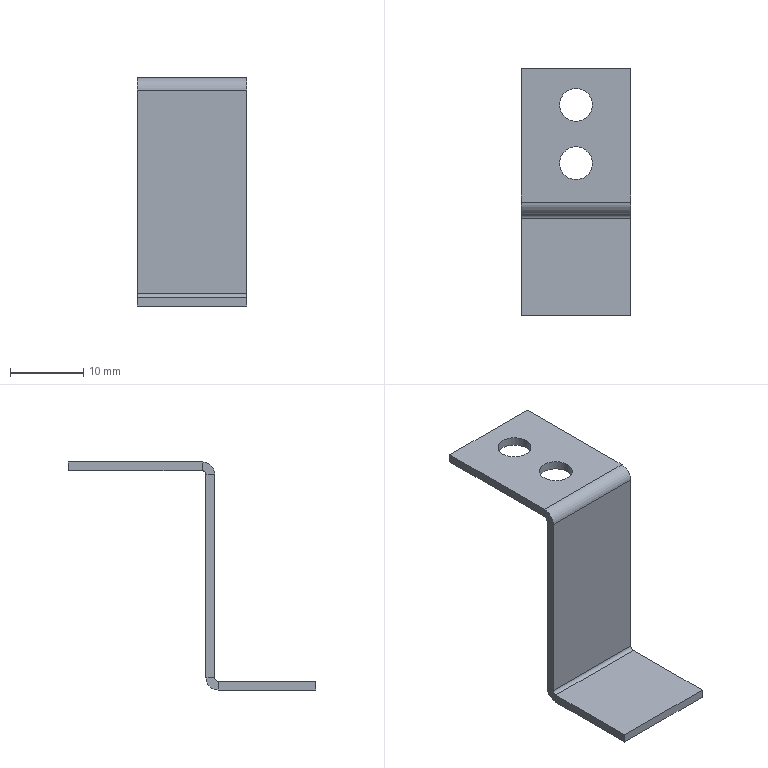Part | SolidWorks | features EdgeFlange 2, FlatPattern 1, HoleWzd 1, SMBaseFlange 1, SheetMetal 1 | 1 solid | 26 faces | box 15 x 33.8 x 31.2 mm | volume 1093 mm3 | plane 18 | cylinder 8 | commonest cylinder face diameters 4.5 x4 1 x2 3.4 x2
STEP:
#1=CARTESIAN_POINT('',(-2.25,5.,-1.2));
#2=VERTEX_POINT('',#1);
#3=CARTESIAN_POINT('',(2.25,5.,-1.2));
#4=VERTEX_POINT('',#3);
#5=CARTESIAN_POINT('',(0.,5.,-1.2));
#6=DIRECTION('',(0.,0.,1.));
#7=DIRECTION('',(1.,0.,0.));
#8=AXIS2_PLACEMENT_3D('',#5,#6,#7);
#9=CIRCLE('',#8,2.25);
#10=EDGE_CURVE('',#2,#4,#9,.T.);
#11=ORIENTED_EDGE('',*,*,#10,.F.);
#12=CARTESIAN_POINT('',(-2.25,5.,0.));
#13=VERTEX_POINT('',#12);
#14=CARTESIAN_POINT('',(-2.25,5.,0.));
#15=DIRECTION('',(0.,0.,1.));
#16=VECTOR('',#15,1000.);
#17=LINE('',#14,#16);
#18=EDGE_CURVE('',#2,#13,#17,.T.);
#19=ORIENTED_EDGE('',*,*,#18,.T.);
#20=CARTESIAN_POINT('',(2.25,5.,0.));
#21=VERTEX_POINT('',#20);
#22=CARTESIAN_POINT('',(0.,5.,0.));
#23=DIRECTION('',(0.,0.,1.));
#24=DIRECTION('',(1.,0.,0.));
#25=AXIS2_PLACEMENT_3D('',#22,#23,#24);
#26=CIRCLE('',#25,2.25);
#27=EDGE_CURVE('',#13,#21,#26,.T.);
#28=ORIENTED_EDGE('',*,*,#27,.T.);
#29=CARTESIAN_POINT('',(2.25,5.,0.));
#30=DIRECTION('',(0.,0.,1.));
#31=VECTOR('',#30,1000.);
#32=LINE('',#29,#31);
#33=EDGE_CURVE('',#4,#21,#32,.T.);
#34=ORIENTED_EDGE('',*,*,#33,.F.);
#35=EDGE_LOOP('',(#11,#19,#28,#34));
#36=FACE_OUTER_BOUND('',#35,.T.);
#37=CARTESIAN_POINT('',(0.,5.,0.));
#38=DIRECTION('',(0.,0.,1.));
#39=DIRECTION('',(1.,0.,0.));
#40=AXIS2_PLACEMENT_3D('',#37,#38,#39);
#41=CYLINDRICAL_SURFACE('',#40,2.25);
#42=ADVANCED_FACE('',(#36),#41,.F.);
#43=CARTESIAN_POINT('',(-2.25,-3.,-1.2));
#44=VERTEX_POINT('',#43);
#45=CARTESIAN_POINT('',(2.25,-3.,-1.2));
#46=VERTEX_POINT('',#45);
#47=CARTESIAN_POINT('',(0.,-3.,-1.2));
#48=DIRECTION('',(0.,0.,1.));
#49=DIRECTION('',(1.,0.,0.));
#50=AXIS2_PLACEMENT_3D('',#47,#48,#49);
#51=CIRCLE('',#50,2.25);
#52=EDGE_CURVE('',#44,#46,#51,.T.);
#53=ORIENTED_EDGE('',*,*,#52,.F.);
#54=CARTESIAN_POINT('',(-2.25,-3.,0.));
#55=VERTEX_POINT('',#54);
#56=CARTESIAN_POINT('',(-2.25,-3.,0.));
#57=DIRECTION('',(0.,0.,1.));
#58=VECTOR('',#57,1000.);
#59=LINE('',#56,#58);
#60=EDGE_CURVE('',#44,#55,#59,.T.);
#61=ORIENTED_EDGE('',*,*,#60,.T.);
#62=CARTESIAN_POINT('',(2.25,-3.,0.));
#63=VERTEX_POINT('',#62);
#64=CARTESIAN_POINT('',(0.,-3.,0.));
#65=DIRECTION('',(0.,0.,1.));
#66=DIRECTION('',(1.,0.,0.));
#67=AXIS2_PLACEMENT_3D('',#64,#65,#66);
#68=CIRCLE('',#67,2.25);
#69=EDGE_CURVE('',#55,#63,#68,.T.);
#70=ORIENTED_EDGE('',*,*,#69,.T.);
#71=CARTESIAN_POINT('',(2.25,-3.,0.));
#72=DIRECTION('',(0.,0.,1.));
#73=VECTOR('',#72,1000.);
#74=LINE('',#71,#73);
#75=EDGE_CURVE('',#46,#63,#74,.T.);
#76=ORIENTED_EDGE('',*,*,#75,.F.);
#77=EDGE_LOOP('',(#53,#61,#70,#76));
#78=FACE_OUTER_BOUND('',#77,.T.);
#79=CARTESIAN_POINT('',(0.,-3.,0.));
#80=DIRECTION('',(0.,0.,1.));
#81=DIRECTION('',(1.,0.,0.));
#82=AXIS2_PLACEMENT_3D('',#79,#80,#81);
#83=CYLINDRICAL_SURFACE('',#82,2.25);
#84=ADVANCED_FACE('',(#78),#83,.F.);
#85=CARTESIAN_POINT('',(-7.5,-10.,-29.5));
#86=VERTEX_POINT('',#85);
#87=CARTESIAN_POINT('',(-7.5,-8.8,-29.5));
#88=VERTEX_POINT('',#87);
#89=CARTESIAN_POINT('',(-7.5,-10.,-29.5));
#90=DIRECTION('',(0.,1.,0.));
#91=VECTOR('',#90,1000.);
#92=LINE('',#89,#91);
#93=EDGE_CURVE('',#86,#88,#92,.T.);
#94=ORIENTED_EDGE('',*,*,#93,.F.);
#95=CARTESIAN_POINT('',(-7.5,-10.,-1.7));
#96=VERTEX_POINT('',#95);
#97=CARTESIAN_POINT('',(-7.5,-10.,0.));
#98=DIRECTION('',(0.,0.,-1.));
#99=VECTOR('',#98,1000.);
#100=LINE('',#97,#99);
#101=EDGE_CURVE('',#96,#86,#100,.T.);
#102=ORIENTED_EDGE('',*,*,#101,.F.);
#103=CARTESIAN_POINT('',(-7.5,-8.8,-1.7));
#104=VERTEX_POINT('',#103);
#105=CARTESIAN_POINT('',(-7.5,-8.8,-1.7));
#106=DIRECTION('',(0.,-1.,0.));
#107=VECTOR('',#106,1000.);
#108=LINE('',#105,#107);
#109=EDGE_CURVE('',#104,#96,#108,.T.);
#110=ORIENTED_EDGE('',*,*,#109,.F.);
#111=CARTESIAN_POINT('',(-7.5,-8.8,-30.));
#112=DIRECTION('',(0.,0.,-1.));
#113=VECTOR('',#112,1000.);
#114=LINE('',#111,#113);
#115=EDGE_CURVE('',#104,#88,#114,.T.);
#116=ORIENTED_EDGE('',*,*,#115,.T.);
#117=EDGE_LOOP('',(#94,#102,#110,#116));
#118=FACE_OUTER_BOUND('',#117,.T.);
#119=CARTESIAN_POINT('',(-7.5,-10.,-30.));
#120=DIRECTION('',(1.,0.,0.));
#121=DIRECTION('',(0.,0.,-1.));
#122=AXIS2_PLACEMENT_3D('',#119,#120,#121);
#123=PLANE('',#122);
#124=ADVANCED_FACE('',(#118),#123,.F.);
#125=CARTESIAN_POINT('',(7.5,-10.,-29.5));
#126=VERTEX_POINT('',#125);
#127=CARTESIAN_POINT('',(7.5,-8.8,-29.5));
#128=VERTEX_POINT('',#127);
#129=CARTESIAN_POINT('',(7.5,-10.,-29.5));
#130=DIRECTION('',(0.,1.,0.));
#131=VECTOR('',#130,1000.);
#132=LINE('',#129,#131);
#133=EDGE_CURVE('',#126,#128,#132,.T.);
#134=ORIENTED_EDGE('',*,*,#133,.T.);
#135=CARTESIAN_POINT('',(7.5,-8.8,-1.7));
#136=VERTEX_POINT('',#135);
#137=CARTESIAN_POINT('',(7.5,-8.8,-1.2));
#138=DIRECTION('',(0.,0.,1.));
#139=VECTOR('',#138,1000.);
#140=LINE('',#137,#139);
#141=EDGE_CURVE('',#128,#136,#140,.T.);
#142=ORIENTED_EDGE('',*,*,#141,.T.);
#143=CARTESIAN_POINT('',(7.5,-10.,-1.7));
#144=VERTEX_POINT('',#143);
#145=CARTESIAN_POINT('',(7.5,-10.,-1.7));
#146=DIRECTION('',(0.,-1.,0.));
#147=VECTOR('',#146,1000.);
#148=LINE('',#145,#147);
#149=EDGE_CURVE('',#136,#144,#148,.T.);
#150=ORIENTED_EDGE('',*,*,#149,.T.);
#151=CARTESIAN_POINT('',(7.5,-10.,0.));
#152=DIRECTION('',(0.,0.,1.));
#153=VECTOR('',#152,1000.);
#154=LINE('',#151,#153);
#155=EDGE_CURVE('',#126,#144,#154,.T.);
#156=ORIENTED_EDGE('',*,*,#155,.F.);
#157=EDGE_LOOP('',(#134,#142,#150,#156));
#158=FACE_OUTER_BOUND('',#157,.T.);
#159=CARTESIAN_POINT('',(7.5,-10.,-1.2));
#160=DIRECTION('',(-1.,0.,0.));
#161=DIRECTION('',(0.,0.,1.));
#162=AXIS2_PLACEMENT_3D('',#159,#160,#161);
#163=PLANE('',#162);
#164=ADVANCED_FACE('',(#158),#163,.F.);
#165=CARTESIAN_POINT('',(7.5,-10.,-29.5));
#166=DIRECTION('',(-1.,0.,0.));
#167=VECTOR('',#166,1000.);
#168=LINE('',#165,#167);
#169=EDGE_CURVE('',#126,#86,#168,.T.);
#170=ORIENTED_EDGE('',*,*,#169,.F.);
#171=ORIENTED_EDGE('',*,*,#155,.T.);
#172=CARTESIAN_POINT('',(7.5,-10.,-1.7));
#173=DIRECTION('',(1.,0.,0.));
#174=VECTOR('',#173,1000.);
#175=LINE('',#172,#174);
#176=EDGE_CURVE('',#96,#144,#175,.T.);
#177=ORIENTED_EDGE('',*,*,#176,.F.);
#178=ORIENTED_EDGE('',*,*,#101,.T.);
#179=EDGE_LOOP('',(#170,#171,#177,#178));
#180=FACE_OUTER_BOUND('',#179,.T.);
#181=CARTESIAN_POINT('',(0.,-10.,0.));
#182=DIRECTION('',(0.,1.,0.));
#183=DIRECTION('',(0.,0.,1.));
#184=AXIS2_PLACEMENT_3D('',#181,#182,#183);
#185=PLANE('',#184);
#186=ADVANCED_FACE('',(#180),#185,.F.);
#187=ORIENTED_EDGE('',*,*,#141,.F.);
#188=CARTESIAN_POINT('',(7.5,-8.8,-29.5));
#189=DIRECTION('',(-1.,0.,0.));
#190=VECTOR('',#189,1000.);
#191=LINE('',#188,#190);
#192=EDGE_CURVE('',#128,#88,#191,.T.);
#193=ORIENTED_EDGE('',*,*,#192,.T.);
#194=ORIENTED_EDGE('',*,*,#115,.F.);
#195=CARTESIAN_POINT('',(7.5,-8.8,-1.7));
#196=DIRECTION('',(-1.,0.,0.));
#197=VECTOR('',#196,1000.);
#198=LINE('',#195,#197);
#199=EDGE_CURVE('',#136,#104,#198,.T.);
#200=ORIENTED_EDGE('',*,*,#199,.F.);
#201=EDGE_LOOP('',(#187,#193,#194,#200));
#202=FACE_OUTER_BOUND('',#201,.T.);
#203=CARTESIAN_POINT('',(0.,-8.8,0.));
#204=DIRECTION('',(0.,1.,0.));
#205=DIRECTION('',(0.,0.,1.));
#206=AXIS2_PLACEMENT_3D('',#203,#204,#205);
#207=PLANE('',#206);
#208=ADVANCED_FACE('',(#202),#207,.T.);
#209=CARTESIAN_POINT('',(-7.5,10.,-1.2));
#210=VERTEX_POINT('',#209);
#211=CARTESIAN_POINT('',(-7.5,-8.3,-1.2));
#212=VERTEX_POINT('',#211);
#213=CARTESIAN_POINT('',(-7.5,-10.,-1.2));
#214=DIRECTION('',(0.,-1.,0.));
#215=VECTOR('',#214,1000.);
#216=LINE('',#213,#215);
#217=EDGE_CURVE('',#210,#212,#216,.T.);
#218=ORIENTED_EDGE('',*,*,#217,.T.);
#219=CARTESIAN_POINT('',(-7.5,-8.3,0.));
#220=VERTEX_POINT('',#219);
#221=CARTESIAN_POINT('',(-7.5,-8.3,-1.2));
#222=DIRECTION('',(0.,0.,1.));
#223=VECTOR('',#222,1000.);
#224=LINE('',#221,#223);
#225=EDGE_CURVE('',#212,#220,#224,.T.);
#226=ORIENTED_EDGE('',*,*,#225,.T.);
#227=CARTESIAN_POINT('',(-7.5,10.,0.));
#228=VERTEX_POINT('',#227);
#229=CARTESIAN_POINT('',(-7.5,-10.,0.));
#230=DIRECTION('',(0.,-1.,0.));
#231=VECTOR('',#230,1000.);
#232=LINE('',#229,#231);
#233=EDGE_CURVE('',#228,#220,#232,.T.);
#234=ORIENTED_EDGE('',*,*,#233,.F.);
#235=CARTESIAN_POINT('',(-7.5,10.,-1.2));
#236=DIRECTION('',(0.,0.,1.));
#237=VECTOR('',#236,1000.);
#238=LINE('',#235,#237);
#239=EDGE_CURVE('',#210,#228,#238,.T.);
#240=ORIENTED_EDGE('',*,*,#239,.F.);
#241=EDGE_LOOP('',(#218,#226,#234,#240));
#242=FACE_OUTER_BOUND('',#241,.T.);
#243=CARTESIAN_POINT('',(-7.5,-10.,-1.2));
#244=DIRECTION('',(-1.,0.,0.));
#245=DIRECTION('',(0.,0.,1.));
#246=AXIS2_PLACEMENT_3D('',#243,#244,#245);
#247=PLANE('',#246);
#248=ADVANCED_FACE('',(#242),#247,.T.);
#249=CARTESIAN_POINT('',(0.,5.,-1.2));
#250=DIRECTION('',(0.,0.,1.));
#251=DIRECTION('',(1.,0.,0.));
#252=AXIS2_PLACEMENT_3D('',#249,#250,#251);
#253=CIRCLE('',#252,2.25);
#254=EDGE_CURVE('',#4,#2,#253,.T.);
#255=ORIENTED_EDGE('',*,*,#254,.T.);
#256=ORIENTED_EDGE('',*,*,#10,.T.);
#257=EDGE_LOOP('',(#255,#256));
#258=FACE_BOUND('',#257,.T.);
#259=CARTESIAN_POINT('',(0.,-3.,-1.2));
#260=DIRECTION('',(0.,0.,1.));
#261=DIRECTION('',(1.,0.,0.));
#262=AXIS2_PLACEMENT_3D('',#259,#260,#261);
#263=CIRCLE('',#262,2.25);
#264=EDGE_CURVE('',#46,#44,#263,.T.);
#265=ORIENTED_EDGE('',*,*,#264,.T.);
#266=ORIENTED_EDGE('',*,*,#52,.T.);
#267=EDGE_LOOP('',(#265,#266));
#268=FACE_BOUND('',#267,.T.);
#269=CARTESIAN_POINT('',(7.5,-8.3,-1.2));
#270=VERTEX_POINT('',#269);
#271=CARTESIAN_POINT('',(7.5,10.,-1.2));
#272=VERTEX_POINT('',#271);
#273=CARTESIAN_POINT('',(7.5,-10.,-1.2));
#274=DIRECTION('',(0.,1.,0.));
#275=VECTOR('',#274,1000.);
#276=LINE('',#273,#275);
#277=EDGE_CURVE('',#270,#272,#276,.T.);
#278=ORIENTED_EDGE('',*,*,#277,.F.);
#279=CARTESIAN_POINT('',(-7.5,-8.3,-1.2));
#280=DIRECTION('',(1.,0.,0.));
#281=VECTOR('',#280,1000.);
#282=LINE('',#279,#281);
#283=EDGE_CURVE('',#212,#270,#282,.T.);
#284=ORIENTED_EDGE('',*,*,#283,.F.);
#285=ORIENTED_EDGE('',*,*,#217,.F.);
#286=CARTESIAN_POINT('',(-7.5,10.,-1.2));
#287=DIRECTION('',(-1.,0.,0.));
#288=VECTOR('',#287,1000.);
#289=LINE('',#286,#288);
#290=EDGE_CURVE('',#272,#210,#289,.T.);
#291=ORIENTED_EDGE('',*,*,#290,.F.);
#292=EDGE_LOOP('',(#278,#284,#285,#291));
#293=FACE_OUTER_BOUND('',#292,.T.);
#294=CARTESIAN_POINT('',(0.,0.,-1.2));
#295=DIRECTION('',(0.,0.,-1.));
#296=DIRECTION('',(-1.,0.,0.));
#297=AXIS2_PLACEMENT_3D('',#294,#295,#296);
#298=PLANE('',#297);
#299=ADVANCED_FACE('',(#258,#268,#293),#298,.T.);
#300=CARTESIAN_POINT('',(0.,-3.,0.));
#301=DIRECTION('',(0.,0.,1.));
#302=DIRECTION('',(1.,0.,0.));
#303=AXIS2_PLACEMENT_3D('',#300,#301,#302);
#304=CIRCLE('',#303,2.25);
#305=EDGE_CURVE('',#63,#55,#304,.T.);
#306=ORIENTED_EDGE('',*,*,#305,.F.);
#307=ORIENTED_EDGE('',*,*,#69,.F.);
#308=EDGE_LOOP('',(#306,#307));
#309=FACE_BOUND('',#308,.T.);
#310=CARTESIAN_POINT('',(0.,5.,0.));
#311=DIRECTION('',(0.,0.,1.));
#312=DIRECTION('',(1.,0.,0.));
#313=AXIS2_PLACEMENT_3D('',#310,#311,#312);
#314=CIRCLE('',#313,2.25);
#315=EDGE_CURVE('',#21,#13,#314,.T.);
#316=ORIENTED_EDGE('',*,*,#315,.F.);
#317=ORIENTED_EDGE('',*,*,#27,.F.);
#318=EDGE_LOOP('',(#316,#317));
#319=FACE_BOUND('',#318,.T.);
#320=CARTESIAN_POINT('',(7.5,-8.3,0.));
#321=VERTEX_POINT('',#320);
#322=CARTESIAN_POINT('',(-7.5,-8.3,0.));
#323=DIRECTION('',(1.,0.,0.));
#324=VECTOR('',#323,1000.);
#325=LINE('',#322,#324);
#326=EDGE_CURVE('',#220,#321,#325,.T.);
#327=ORIENTED_EDGE('',*,*,#326,.T.);
#328=CARTESIAN_POINT('',(7.5,10.,0.));
#329=VERTEX_POINT('',#328);
#330=CARTESIAN_POINT('',(7.5,-10.,0.));
#331=DIRECTION('',(0.,1.,0.));
#332=VECTOR('',#331,1000.);
#333=LINE('',#330,#332);
#334=EDGE_CURVE('',#321,#329,#333,.T.);
#335=ORIENTED_EDGE('',*,*,#334,.T.);
#336=CARTESIAN_POINT('',(-7.5,10.,0.));
#337=DIRECTION('',(-1.,0.,0.));
#338=VECTOR('',#337,1000.);
#339=LINE('',#336,#338);
#340=EDGE_CURVE('',#329,#228,#339,.T.);
#341=ORIENTED_EDGE('',*,*,#340,.T.);
#342=ORIENTED_EDGE('',*,*,#233,.T.);
#343=EDGE_LOOP('',(#327,#335,#341,#342));
#344=FACE_OUTER_BOUND('',#343,.T.);
#345=CARTESIAN_POINT('',(0.,0.,0.));
#346=DIRECTION('',(0.,0.,-1.));
#347=DIRECTION('',(-1.,0.,0.));
#348=AXIS2_PLACEMENT_3D('',#345,#346,#347);
#349=PLANE('',#348);
#350=ADVANCED_FACE('',(#309,#319,#344),#349,.F.);
#351=CARTESIAN_POINT('',(7.5,-8.3,-1.2));
#352=DIRECTION('',(0.,0.,1.));
#353=VECTOR('',#352,1000.);
#354=LINE('',#351,#353);
#355=EDGE_CURVE('',#270,#321,#354,.T.);
#356=ORIENTED_EDGE('',*,*,#355,.F.);
#357=ORIENTED_EDGE('',*,*,#277,.T.);
#358=CARTESIAN_POINT('',(7.5,10.,-1.2));
#359=DIRECTION('',(0.,0.,1.));
#360=VECTOR('',#359,1000.);
#361=LINE('',#358,#360);
#362=EDGE_CURVE('',#272,#329,#361,.T.);
#363=ORIENTED_EDGE('',*,*,#362,.T.);
#364=ORIENTED_EDGE('',*,*,#334,.F.);
#365=EDGE_LOOP('',(#356,#357,#363,#364));
#366=FACE_OUTER_BOUND('',#365,.T.);
#367=CARTESIAN_POINT('',(7.5,-10.,-1.2));
#368=DIRECTION('',(1.,0.,0.));
#369=DIRECTION('',(0.,0.,-1.));
#370=AXIS2_PLACEMENT_3D('',#367,#368,#369);
#371=PLANE('',#370);
#372=ADVANCED_FACE('',(#366),#371,.T.);
#373=ORIENTED_EDGE('',*,*,#340,.F.);
#374=ORIENTED_EDGE('',*,*,#362,.F.);
#375=ORIENTED_EDGE('',*,*,#290,.T.);
#376=ORIENTED_EDGE('',*,*,#239,.T.);
#377=EDGE_LOOP('',(#373,#374,#375,#376));
#378=FACE_OUTER_BOUND('',#377,.T.);
#379=CARTESIAN_POINT('',(-7.5,10.,-1.2));
#380=DIRECTION('',(0.,1.,0.));
#381=DIRECTION('',(0.,0.,1.));
#382=AXIS2_PLACEMENT_3D('',#379,#380,#381);
#383=PLANE('',#382);
#384=ADVANCED_FACE('',(#378),#383,.T.);
#385=ORIENTED_EDGE('',*,*,#60,.F.);
#386=ORIENTED_EDGE('',*,*,#264,.F.);
#387=ORIENTED_EDGE('',*,*,#75,.T.);
#388=ORIENTED_EDGE('',*,*,#305,.T.);
#389=EDGE_LOOP('',(#385,#386,#387,#388));
#390=FACE_OUTER_BOUND('',#389,.T.);
#391=CARTESIAN_POINT('',(0.,-3.,0.));
#392=DIRECTION('',(0.,0.,1.));
#393=DIRECTION('',(1.,0.,0.));
#394=AXIS2_PLACEMENT_3D('',#391,#392,#393);
#395=CYLINDRICAL_SURFACE('',#394,2.25);
#396=ADVANCED_FACE('',(#390),#395,.F.);
#397=ORIENTED_EDGE('',*,*,#18,.F.);
#398=ORIENTED_EDGE('',*,*,#254,.F.);
#399=ORIENTED_EDGE('',*,*,#33,.T.);
#400=ORIENTED_EDGE('',*,*,#315,.T.);
#401=EDGE_LOOP('',(#397,#398,#399,#400));
#402=FACE_OUTER_BOUND('',#401,.T.);
#403=CARTESIAN_POINT('',(0.,5.,0.));
#404=DIRECTION('',(0.,0.,1.));
#405=DIRECTION('',(1.,0.,0.));
#406=AXIS2_PLACEMENT_3D('',#403,#404,#405);
#407=CYLINDRICAL_SURFACE('',#406,2.25);
#408=ADVANCED_FACE('',(#402),#407,.F.);
#409=ORIENTED_EDGE('',*,*,#149,.F.);
#410=CARTESIAN_POINT('',(7.5,-8.3,-1.7));
#411=DIRECTION('',(1.,0.,0.));
#412=DIRECTION('',(0.,0.,1.));
#413=AXIS2_PLACEMENT_3D('',#410,#411,#412);
#414=CIRCLE('',#413,0.5);
#415=EDGE_CURVE('',#270,#136,#414,.T.);
#416=ORIENTED_EDGE('',*,*,#415,.F.);
#417=ORIENTED_EDGE('',*,*,#355,.T.);
#418=CARTESIAN_POINT('',(7.5,-8.3,-1.7));
#419=DIRECTION('',(1.,0.,0.));
#420=DIRECTION('',(0.,0.,1.));
#421=AXIS2_PLACEMENT_3D('',#418,#419,#420);
#422=CIRCLE('',#421,1.7);
#423=EDGE_CURVE('',#321,#144,#422,.T.);
#424=ORIENTED_EDGE('',*,*,#423,.T.);
#425=EDGE_LOOP('',(#409,#416,#417,#424));
#426=FACE_OUTER_BOUND('',#425,.T.);
#427=CARTESIAN_POINT('',(7.5,-8.3,-1.7));
#428=DIRECTION('',(1.,0.,0.));
#429=DIRECTION('',(0.,0.,-1.));
#430=AXIS2_PLACEMENT_3D('',#427,#428,#429);
#431=PLANE('',#430);
#432=ADVANCED_FACE('',(#426),#431,.T.);
#433=CARTESIAN_POINT('',(-7.5,-8.3,-1.7));
#434=DIRECTION('',(-1.,0.,0.));
#435=DIRECTION('',(0.,0.,1.));
#436=AXIS2_PLACEMENT_3D('',#433,#434,#435);
#437=CIRCLE('',#436,0.5);
#438=EDGE_CURVE('',#104,#212,#437,.T.);
#439=ORIENTED_EDGE('',*,*,#438,.F.);
#440=ORIENTED_EDGE('',*,*,#109,.T.);
#441=CARTESIAN_POINT('',(-7.5,-8.3,-1.7));
#442=DIRECTION('',(-1.,0.,0.));
#443=DIRECTION('',(0.,0.,1.));
#444=AXIS2_PLACEMENT_3D('',#441,#442,#443);
#445=CIRCLE('',#444,1.7);
#446=EDGE_CURVE('',#96,#220,#445,.T.);
#447=ORIENTED_EDGE('',*,*,#446,.T.);
#448=ORIENTED_EDGE('',*,*,#225,.F.);
#449=EDGE_LOOP('',(#439,#440,#447,#448));
#450=FACE_OUTER_BOUND('',#449,.T.);
#451=CARTESIAN_POINT('',(-7.5,-8.3,-1.7));
#452=DIRECTION('',(1.,0.,0.));
#453=DIRECTION('',(0.,0.,-1.));
#454=AXIS2_PLACEMENT_3D('',#451,#452,#453);
#455=PLANE('',#454);
#456=ADVANCED_FACE('',(#450),#455,.F.);
#457=ORIENTED_EDGE('',*,*,#326,.F.);
#458=ORIENTED_EDGE('',*,*,#446,.F.);
#459=ORIENTED_EDGE('',*,*,#176,.T.);
#460=ORIENTED_EDGE('',*,*,#423,.F.);
#461=EDGE_LOOP('',(#457,#458,#459,#460));
#462=FACE_OUTER_BOUND('',#461,.T.);
#463=CARTESIAN_POINT('',(-7.5,-8.3,-1.7));
#464=DIRECTION('',(-1.,0.,0.));
#465=DIRECTION('',(0.,-1.,0.));
#466=AXIS2_PLACEMENT_3D('',#463,#464,#465);
#467=CYLINDRICAL_SURFACE('',#466,1.7);
#468=ADVANCED_FACE('',(#462),#467,.T.);
#469=ORIENTED_EDGE('',*,*,#283,.T.);
#470=ORIENTED_EDGE('',*,*,#415,.T.);
#471=ORIENTED_EDGE('',*,*,#199,.T.);
#472=ORIENTED_EDGE('',*,*,#438,.T.);
#473=EDGE_LOOP('',(#469,#470,#471,#472));
#474=FACE_OUTER_BOUND('',#473,.T.);
#475=CARTESIAN_POINT('',(-7.5,-8.3,-1.7));
#476=DIRECTION('',(-1.,0.,0.));
#477=DIRECTION('',(0.,-1.,0.));
#478=AXIS2_PLACEMENT_3D('',#475,#476,#477);
#479=CYLINDRICAL_SURFACE('',#478,0.5);
#480=ADVANCED_FACE('',(#474),#479,.F.);
#481=CARTESIAN_POINT('',(-7.5,-10.5,-30.));
#482=VERTEX_POINT('',#481);
#483=CARTESIAN_POINT('',(-7.5,-10.5,-31.2));
#484=VERTEX_POINT('',#483);
#485=CARTESIAN_POINT('',(-7.5,-10.5,-30.));
#486=DIRECTION('',(0.,0.,-1.));
#487=VECTOR('',#486,1000.);
#488=LINE('',#485,#487);
#489=EDGE_CURVE('',#482,#484,#488,.T.);
#490=ORIENTED_EDGE('',*,*,#489,.F.);
#491=CARTESIAN_POINT('',(-7.5,-10.5,-29.5));
#492=DIRECTION('',(-1.,0.,0.));
#493=DIRECTION('',(0.,0.,-1.));
#494=AXIS2_PLACEMENT_3D('',#491,#492,#493);
#495=CIRCLE('',#494,0.5);
#496=EDGE_CURVE('',#86,#482,#495,.T.);
#497=ORIENTED_EDGE('',*,*,#496,.F.);
#498=ORIENTED_EDGE('',*,*,#93,.T.);
#499=CARTESIAN_POINT('',(-7.5,-10.5,-29.5));
#500=DIRECTION('',(-1.,0.,0.));
#501=DIRECTION('',(0.,0.,-1.));
#502=AXIS2_PLACEMENT_3D('',#499,#500,#501);
#503=CIRCLE('',#502,1.7);
#504=EDGE_CURVE('',#88,#484,#503,.T.);
#505=ORIENTED_EDGE('',*,*,#504,.T.);
#506=EDGE_LOOP('',(#490,#497,#498,#505));
#507=FACE_OUTER_BOUND('',#506,.T.);
#508=CARTESIAN_POINT('',(-7.5,-10.5,-29.5));
#509=DIRECTION('',(-1.,0.,0.));
#510=DIRECTION('',(0.,0.,1.));
#511=AXIS2_PLACEMENT_3D('',#508,#509,#510);
#512=PLANE('',#511);
#513=ADVANCED_FACE('',(#507),#512,.T.);
#514=CARTESIAN_POINT('',(7.5,-10.5,-30.));
#515=VERTEX_POINT('',#514);
#516=CARTESIAN_POINT('',(7.5,-10.5,-29.5));
#517=DIRECTION('',(1.,0.,0.));
#518=DIRECTION('',(0.,0.,-1.));
#519=AXIS2_PLACEMENT_3D('',#516,#517,#518);
#520=CIRCLE('',#519,0.5);
#521=EDGE_CURVE('',#515,#126,#520,.T.);
#522=ORIENTED_EDGE('',*,*,#521,.F.);
#523=CARTESIAN_POINT('',(7.5,-10.5,-31.2));
#524=VERTEX_POINT('',#523);
#525=CARTESIAN_POINT('',(7.5,-10.5,-30.));
#526=DIRECTION('',(0.,0.,-1.));
#527=VECTOR('',#526,1000.);
#528=LINE('',#525,#527);
#529=EDGE_CURVE('',#515,#524,#528,.T.);
#530=ORIENTED_EDGE('',*,*,#529,.T.);
#531=CARTESIAN_POINT('',(7.5,-10.5,-29.5));
#532=DIRECTION('',(1.,0.,0.));
#533=DIRECTION('',(0.,0.,-1.));
#534=AXIS2_PLACEMENT_3D('',#531,#532,#533);
#535=CIRCLE('',#534,1.7);
#536=EDGE_CURVE('',#524,#128,#535,.T.);
#537=ORIENTED_EDGE('',*,*,#536,.T.);
#538=ORIENTED_EDGE('',*,*,#133,.F.);
#539=EDGE_LOOP('',(#522,#530,#537,#538));
#540=FACE_OUTER_BOUND('',#539,.T.);
#541=CARTESIAN_POINT('',(7.5,-10.5,-29.5));
#542=DIRECTION('',(-1.,0.,0.));
#543=DIRECTION('',(0.,0.,1.));
#544=AXIS2_PLACEMENT_3D('',#541,#542,#543);
#545=PLANE('',#544);
#546=ADVANCED_FACE('',(#540),#545,.F.);
#547=ORIENTED_EDGE('',*,*,#192,.F.);
#548=ORIENTED_EDGE('',*,*,#536,.F.);
#549=CARTESIAN_POINT('',(0.,-10.5,-31.2));
#550=DIRECTION('',(1.,0.,0.));
#551=VECTOR('',#550,1000.);
#552=LINE('',#549,#551);
#553=EDGE_CURVE('',#484,#524,#552,.T.);
#554=ORIENTED_EDGE('',*,*,#553,.F.);
#555=ORIENTED_EDGE('',*,*,#504,.F.);
#556=EDGE_LOOP('',(#547,#548,#554,#555));
#557=FACE_OUTER_BOUND('',#556,.T.);
#558=CARTESIAN_POINT('',(7.5,-10.5,-29.5));
#559=DIRECTION('',(1.,0.,0.));
#560=DIRECTION('',(0.,0.,-1.));
#561=AXIS2_PLACEMENT_3D('',#558,#559,#560);
#562=CYLINDRICAL_SURFACE('',#561,1.7);
#563=ADVANCED_FACE('',(#557),#562,.T.);
#564=ORIENTED_EDGE('',*,*,#169,.T.);
#565=ORIENTED_EDGE('',*,*,#496,.T.);
#566=CARTESIAN_POINT('',(-7.5,-10.5,-30.));
#567=DIRECTION('',(1.,0.,0.));
#568=VECTOR('',#567,1000.);
#569=LINE('',#566,#568);
#570=EDGE_CURVE('',#482,#515,#569,.T.);
#571=ORIENTED_EDGE('',*,*,#570,.T.);
#572=ORIENTED_EDGE('',*,*,#521,.T.);
#573=EDGE_LOOP('',(#564,#565,#571,#572));
#574=FACE_OUTER_BOUND('',#573,.T.);
#575=CARTESIAN_POINT('',(7.5,-10.5,-29.5));
#576=DIRECTION('',(1.,0.,0.));
#577=DIRECTION('',(0.,0.,-1.));
#578=AXIS2_PLACEMENT_3D('',#575,#576,#577);
#579=CYLINDRICAL_SURFACE('',#578,0.5);
#580=ADVANCED_FACE('',(#574),#579,.F.);
#581=CARTESIAN_POINT('',(7.5,-23.8,-31.2));
#582=VERTEX_POINT('',#581);
#583=CARTESIAN_POINT('',(7.5,-10.,-31.2));
#584=DIRECTION('',(0.,1.,0.));
#585=VECTOR('',#584,1000.);
#586=LINE('',#583,#585);
#587=EDGE_CURVE('',#582,#524,#586,.T.);
#588=ORIENTED_EDGE('',*,*,#587,.T.);
#589=ORIENTED_EDGE('',*,*,#529,.F.);
#590=CARTESIAN_POINT('',(7.5,-23.8,-30.));
#591=VERTEX_POINT('',#590);
#592=CARTESIAN_POINT('',(7.5,-10.,-30.));
#593=DIRECTION('',(0.,1.,0.));
#594=VECTOR('',#593,1000.);
#595=LINE('',#592,#594);
#596=EDGE_CURVE('',#591,#515,#595,.T.);
#597=ORIENTED_EDGE('',*,*,#596,.F.);
#598=CARTESIAN_POINT('',(7.5,-23.8,-31.2));
#599=DIRECTION('',(0.,0.,1.));
#600=VECTOR('',#599,1000.);
#601=LINE('',#598,#600);
#602=EDGE_CURVE('',#582,#591,#601,.T.);
#603=ORIENTED_EDGE('',*,*,#602,.F.);
#604=EDGE_LOOP('',(#588,#589,#597,#603));
#605=FACE_OUTER_BOUND('',#604,.T.);
#606=CARTESIAN_POINT('',(7.5,-10.,-31.2));
#607=DIRECTION('',(1.,0.,0.));
#608=DIRECTION('',(0.,1.,0.));
#609=AXIS2_PLACEMENT_3D('',#606,#607,#608);
#610=PLANE('',#609);
#611=ADVANCED_FACE('',(#605),#610,.T.);
#612=CARTESIAN_POINT('',(-7.5,-23.8,-30.));
#613=VERTEX_POINT('',#612);
#614=CARTESIAN_POINT('',(-7.5,-23.8,-30.));
#615=DIRECTION('',(0.,-1.,0.));
#616=VECTOR('',#615,1000.);
#617=LINE('',#614,#616);
#618=EDGE_CURVE('',#482,#613,#617,.T.);
#619=ORIENTED_EDGE('',*,*,#618,.F.);
#620=ORIENTED_EDGE('',*,*,#489,.T.);
#621=CARTESIAN_POINT('',(-7.5,-23.8,-31.2));
#622=VERTEX_POINT('',#621);
#623=CARTESIAN_POINT('',(-7.5,-23.8,-31.2));
#624=DIRECTION('',(0.,-1.,0.));
#625=VECTOR('',#624,1000.);
#626=LINE('',#623,#625);
#627=EDGE_CURVE('',#484,#622,#626,.T.);
#628=ORIENTED_EDGE('',*,*,#627,.T.);
#629=CARTESIAN_POINT('',(-7.5,-23.8,-31.2));
#630=DIRECTION('',(0.,0.,1.));
#631=VECTOR('',#630,1000.);
#632=LINE('',#629,#631);
#633=EDGE_CURVE('',#622,#613,#632,.T.);
#634=ORIENTED_EDGE('',*,*,#633,.T.);
#635=EDGE_LOOP('',(#619,#620,#628,#634));
#636=FACE_OUTER_BOUND('',#635,.T.);
#637=CARTESIAN_POINT('',(-7.5,-23.8,-31.2));
#638=DIRECTION('',(-1.,0.,0.));
#639=DIRECTION('',(0.,-1.,0.));
#640=AXIS2_PLACEMENT_3D('',#637,#638,#639);
#641=PLANE('',#640);
#642=ADVANCED_FACE('',(#636),#641,.T.);
#643=ORIENTED_EDGE('',*,*,#627,.F.);
#644=ORIENTED_EDGE('',*,*,#553,.T.);
#645=ORIENTED_EDGE('',*,*,#587,.F.);
#646=CARTESIAN_POINT('',(7.5,-23.8,-31.2));
#647=DIRECTION('',(1.,0.,0.));
#648=VECTOR('',#647,1000.);
#649=LINE('',#646,#648);
#650=EDGE_CURVE('',#622,#582,#649,.T.);
#651=ORIENTED_EDGE('',*,*,#650,.F.);
#652=EDGE_LOOP('',(#643,#644,#645,#651));
#653=FACE_OUTER_BOUND('',#652,.T.);
#654=CARTESIAN_POINT('',(0.,0.,-31.2));
#655=DIRECTION('',(0.,0.,-1.));
#656=DIRECTION('',(-1.,0.,0.));
#657=AXIS2_PLACEMENT_3D('',#654,#655,#656);
#658=PLANE('',#657);
#659=ADVANCED_FACE('',(#653),#658,.T.);
#660=ORIENTED_EDGE('',*,*,#570,.F.);
#661=ORIENTED_EDGE('',*,*,#618,.T.);
#662=CARTESIAN_POINT('',(7.5,-23.8,-30.));
#663=DIRECTION('',(1.,0.,0.));
#664=VECTOR('',#663,1000.);
#665=LINE('',#662,#664);
#666=EDGE_CURVE('',#613,#591,#665,.T.);
#667=ORIENTED_EDGE('',*,*,#666,.T.);
#668=ORIENTED_EDGE('',*,*,#596,.T.);
#669=EDGE_LOOP('',(#660,#661,#667,#668));
#670=FACE_OUTER_BOUND('',#669,.T.);
#671=CARTESIAN_POINT('',(0.,0.,-30.));
#672=DIRECTION('',(0.,0.,-1.));
#673=DIRECTION('',(-1.,0.,0.));
#674=AXIS2_PLACEMENT_3D('',#671,#672,#673);
#675=PLANE('',#674);
#676=ADVANCED_FACE('',(#670),#675,.F.);
#677=ORIENTED_EDGE('',*,*,#666,.F.);
#678=ORIENTED_EDGE('',*,*,#633,.F.);
#679=ORIENTED_EDGE('',*,*,#650,.T.);
#680=ORIENTED_EDGE('',*,*,#602,.T.);
#681=EDGE_LOOP('',(#677,#678,#679,#680));
#682=FACE_OUTER_BOUND('',#681,.T.);
#683=CARTESIAN_POINT('',(7.5,-23.8,-31.2));
#684=DIRECTION('',(0.,-1.,0.));
#685=DIRECTION('',(0.,0.,-1.));
#686=AXIS2_PLACEMENT_3D('',#683,#684,#685);
#687=PLANE('',#686);
#688=ADVANCED_FACE('',(#682),#687,.T.);
#689=CLOSED_SHELL('',(#42,#84,#124,#164,#186,#208,#248,#299,#350,#372,#384,#396,#408,#432,#456,#468,#480,#513,#546,#563,#580,#611,#642,#659,#676,#688));
#690=MANIFOLD_SOLID_BREP('',#689);
#691=CARTESIAN_POINT('',(0.,0.,0.));
#692=DIRECTION('',(0.,0.,1.));
#693=DIRECTION('',(1.,0.,0.));
#694=AXIS2_PLACEMENT_3D('',#691,#692,#693);
#695=(LENGTH_UNIT()NAMED_UNIT(*)SI_UNIT(.MILLI.,.METRE.));
#696=UNCERTAINTY_MEASURE_WITH_UNIT(LENGTH_MEASURE(0.00001),#695,'','');
#697=(NAMED_UNIT(*)PLANE_ANGLE_UNIT()SI_UNIT($,.RADIAN.));
#698=(NAMED_UNIT(*)SI_UNIT($,.STERADIAN.)SOLID_ANGLE_UNIT());
#699=(GEOMETRIC_REPRESENTATION_CONTEXT(3)GLOBAL_UNCERTAINTY_ASSIGNED_CONTEXT((#696))GLOBAL_UNIT_ASSIGNED_CONTEXT((#695,#697,#698))REPRESENTATION_CONTEXT('',''));
#700=ADVANCED_BREP_SHAPE_REPRESENTATION('',(#690,#694),#699);